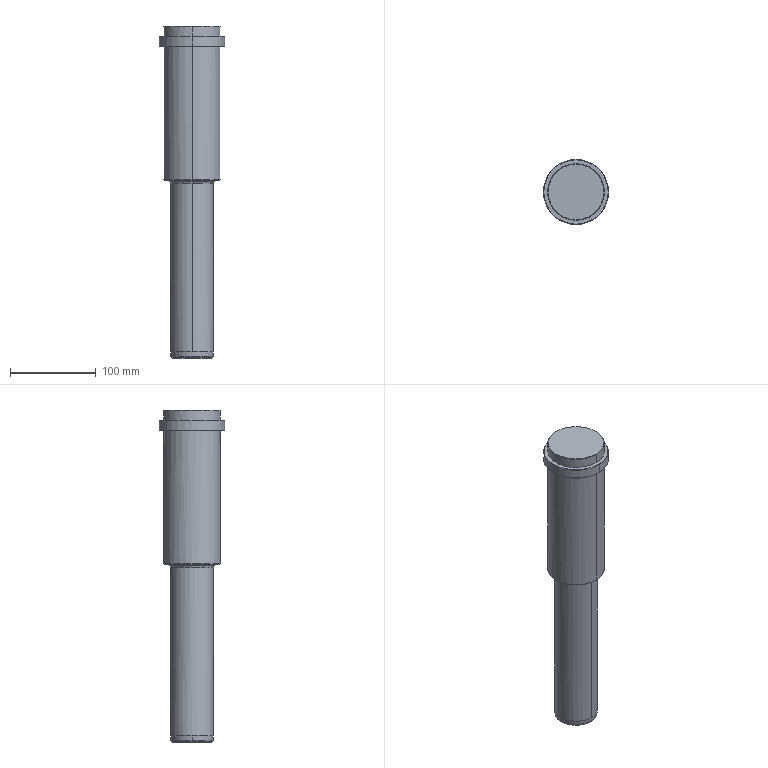Part | Creo | 1 solid | 31 faces | box 76 x 76 x 387 mm | volume 1035650 mm3 | cone 10 | cylinder 8 | torus 8 | plane 5 | commonest cylinder face diameters 66 x4 50 x2 76 x2
STEP:
#1=CARTESIAN_POINT('',(255.,259.495,177.));
#2=VERTEX_POINT('',#1);
#3=CARTESIAN_POINT('',(287.5,291.995,177.));
#4=VERTEX_POINT('',#3);
#5=CARTESIAN_POINT('',(255.,291.995,177.));
#6=DIRECTION('',(0.,0.,1.));
#7=DIRECTION('',(0.,-1.,0.));
#8=AXIS2_PLACEMENT_3D('',#5,#6,#7);
#9=CIRCLE('',#8,32.5);
#10=EDGE_CURVE('',#2,#4,#9,.T.);
#11=ORIENTED_EDGE('',*,*,#10,.F.);
#12=CARTESIAN_POINT('',(222.5,291.995,177.));
#13=VERTEX_POINT('',#12);
#14=CARTESIAN_POINT('',(255.,291.995,177.));
#15=DIRECTION('',(0.,0.,1.));
#16=DIRECTION('',(-1.,0.,0.));
#17=AXIS2_PLACEMENT_3D('',#14,#15,#16);
#18=CIRCLE('',#17,32.5);
#19=EDGE_CURVE('',#13,#2,#18,.T.);
#20=ORIENTED_EDGE('',*,*,#19,.F.);
#21=CARTESIAN_POINT('',(255.,324.495,177.));
#22=VERTEX_POINT('',#21);
#23=CARTESIAN_POINT('',(255.,291.995,177.));
#24=DIRECTION('',(0.,0.,1.));
#25=DIRECTION('',(0.,1.,0.));
#26=AXIS2_PLACEMENT_3D('',#23,#24,#25);
#27=CIRCLE('',#26,32.5);
#28=EDGE_CURVE('',#22,#13,#27,.T.);
#29=ORIENTED_EDGE('',*,*,#28,.F.);
#30=CARTESIAN_POINT('',(255.,291.995,177.));
#31=DIRECTION('',(0.,0.,1.));
#32=DIRECTION('',(1.,0.,0.));
#33=AXIS2_PLACEMENT_3D('',#30,#31,#32);
#34=CIRCLE('',#33,32.5);
#35=EDGE_CURVE('',#4,#22,#34,.T.);
#36=ORIENTED_EDGE('',*,*,#35,.F.);
#37=EDGE_LOOP('',(#11,#20,#29,#36));
#38=FACE_OUTER_BOUND('',#37,.F.);
#39=CARTESIAN_POINT('',(65.,43.995,177.));
#40=DIRECTION('',(0.,0.,1.));
#41=DIRECTION('',(0.,-1.,0.));
#42=AXIS2_PLACEMENT_3D('',#39,#40,#41);
#43=PLANE('',#42);
#44=ADVANCED_FACE('',(#38),#43,.T.);
#45=CARTESIAN_POINT('',(255.,258.995,176.5));
#46=VERTEX_POINT('',#45);
#47=CARTESIAN_POINT('',(288.,291.995,176.5));
#48=VERTEX_POINT('',#47);
#49=CARTESIAN_POINT('',(255.,291.995,176.5));
#50=DIRECTION('',(0.,0.,1.));
#51=DIRECTION('',(0.,-1.,0.));
#52=AXIS2_PLACEMENT_3D('',#49,#50,#51);
#53=CIRCLE('',#52,33.);
#54=EDGE_CURVE('',#46,#48,#53,.T.);
#55=ORIENTED_EDGE('',*,*,#54,.F.);
#56=CARTESIAN_POINT('',(222.,291.995,176.5));
#57=VERTEX_POINT('',#56);
#58=CARTESIAN_POINT('',(255.,291.995,176.5));
#59=DIRECTION('',(0.,0.,1.));
#60=DIRECTION('',(-1.,0.,0.));
#61=AXIS2_PLACEMENT_3D('',#58,#59,#60);
#62=CIRCLE('',#61,33.);
#63=EDGE_CURVE('',#57,#46,#62,.T.);
#64=ORIENTED_EDGE('',*,*,#63,.F.);
#65=CARTESIAN_POINT('',(222.5,291.995,177.));
#66=DIRECTION('',(-0.7071,0.,-0.7071));
#67=VECTOR('',#66,0.7071);
#68=LINE('',#65,#67);
#69=EDGE_CURVE('',#13,#57,#68,.T.);
#70=ORIENTED_EDGE('',*,*,#69,.F.);
#71=ORIENTED_EDGE('',*,*,#19,.T.);
#72=ORIENTED_EDGE('',*,*,#10,.T.);
#73=CARTESIAN_POINT('',(287.5,291.995,177.));
#74=DIRECTION('',(0.7071,0.,-0.7071));
#75=VECTOR('',#74,0.7071);
#76=LINE('',#73,#75);
#77=EDGE_CURVE('',#4,#48,#76,.T.);
#78=ORIENTED_EDGE('',*,*,#77,.T.);
#79=EDGE_LOOP('',(#55,#64,#70,#71,#72,#78));
#80=FACE_OUTER_BOUND('',#79,.F.);
#81=CARTESIAN_POINT('',(255.,291.995,176.75));
#82=DIRECTION('',(0.,0.,-1.));
#83=DIRECTION('',(-1.,0.,0.));
#84=AXIS2_PLACEMENT_3D('',#81,#82,#83);
#85=CONICAL_SURFACE('',#84,32.75,45.);
#86=ADVANCED_FACE('',(#80),#85,.T.);
#87=CARTESIAN_POINT('',(255.,324.995,176.5));
#88=VERTEX_POINT('',#87);
#89=CARTESIAN_POINT('',(255.,291.995,176.5));
#90=DIRECTION('',(0.,0.,1.));
#91=DIRECTION('',(1.,0.,0.));
#92=AXIS2_PLACEMENT_3D('',#89,#90,#91);
#93=CIRCLE('',#92,33.);
#94=EDGE_CURVE('',#48,#88,#93,.T.);
#95=ORIENTED_EDGE('',*,*,#94,.T.);
#96=CARTESIAN_POINT('',(255.,324.995,165.));
#97=VERTEX_POINT('',#96);
#98=CARTESIAN_POINT('',(255.,324.995,165.));
#99=DIRECTION('',(0.,0.,1.));
#100=VECTOR('',#99,11.5);
#101=LINE('',#98,#100);
#102=EDGE_CURVE('',#97,#88,#101,.T.);
#103=ORIENTED_EDGE('',*,*,#102,.F.);
#104=CARTESIAN_POINT('',(255.,258.995,165.));
#105=VERTEX_POINT('',#104);
#106=CARTESIAN_POINT('',(255.,291.995,165.));
#107=DIRECTION('',(0.,0.,-1.));
#108=DIRECTION('',(0.,1.,0.));
#109=AXIS2_PLACEMENT_3D('',#106,#107,#108);
#110=CIRCLE('',#109,33.);
#111=EDGE_CURVE('',#97,#105,#110,.T.);
#112=ORIENTED_EDGE('',*,*,#111,.T.);
#113=CARTESIAN_POINT('',(255.,258.995,165.));
#114=DIRECTION('',(0.,0.,1.));
#115=VECTOR('',#114,11.5);
#116=LINE('',#113,#115);
#117=EDGE_CURVE('',#105,#46,#116,.T.);
#118=ORIENTED_EDGE('',*,*,#117,.T.);
#119=ORIENTED_EDGE('',*,*,#54,.T.);
#120=EDGE_LOOP('',(#95,#103,#112,#118,#119));
#121=FACE_OUTER_BOUND('',#120,.F.);
#122=CARTESIAN_POINT('',(255.,291.995,165.));
#123=DIRECTION('',(0.,0.,1.));
#124=DIRECTION('',(0.,-1.,0.));
#125=AXIS2_PLACEMENT_3D('',#122,#123,#124);
#126=CYLINDRICAL_SURFACE('',#125,33.);
#127=ADVANCED_FACE('',(#121),#126,.T.);
#128=ORIENTED_EDGE('',*,*,#94,.F.);
#129=ORIENTED_EDGE('',*,*,#77,.F.);
#130=ORIENTED_EDGE('',*,*,#35,.T.);
#131=ORIENTED_EDGE('',*,*,#28,.T.);
#132=ORIENTED_EDGE('',*,*,#69,.T.);
#133=CARTESIAN_POINT('',(255.,291.995,176.5));
#134=DIRECTION('',(0.,0.,1.));
#135=DIRECTION('',(0.,1.,0.));
#136=AXIS2_PLACEMENT_3D('',#133,#134,#135);
#137=CIRCLE('',#136,33.);
#138=EDGE_CURVE('',#88,#57,#137,.T.);
#139=ORIENTED_EDGE('',*,*,#138,.F.);
#140=EDGE_LOOP('',(#128,#129,#130,#131,#132,#139));
#141=FACE_OUTER_BOUND('',#140,.F.);
#142=CARTESIAN_POINT('',(255.,291.995,176.75));
#143=DIRECTION('',(0.,0.,-1.));
#144=DIRECTION('',(-1.,0.,0.));
#145=AXIS2_PLACEMENT_3D('',#142,#143,#144);
#146=CONICAL_SURFACE('',#145,32.75,45.);
#147=ADVANCED_FACE('',(#141),#146,.T.);
#148=ORIENTED_EDGE('',*,*,#63,.T.);
#149=ORIENTED_EDGE('',*,*,#117,.F.);
#150=CARTESIAN_POINT('',(255.,291.995,165.));
#151=DIRECTION('',(0.,0.,-1.));
#152=DIRECTION('',(0.,-1.,0.));
#153=AXIS2_PLACEMENT_3D('',#150,#151,#152);
#154=CIRCLE('',#153,33.);
#155=EDGE_CURVE('',#105,#97,#154,.T.);
#156=ORIENTED_EDGE('',*,*,#155,.T.);
#157=ORIENTED_EDGE('',*,*,#102,.T.);
#158=ORIENTED_EDGE('',*,*,#138,.T.);
#159=EDGE_LOOP('',(#148,#149,#156,#157,#158));
#160=FACE_OUTER_BOUND('',#159,.F.);
#161=CARTESIAN_POINT('',(255.,291.995,165.));
#162=DIRECTION('',(0.,0.,1.));
#163=DIRECTION('',(0.,-1.,0.));
#164=AXIS2_PLACEMENT_3D('',#161,#162,#163);
#165=CYLINDRICAL_SURFACE('',#164,33.);
#166=ADVANCED_FACE('',(#160),#165,.T.);
#167=CARTESIAN_POINT('',(255.,254.495,165.));
#168=VERTEX_POINT('',#167);
#169=CARTESIAN_POINT('',(292.5,291.995,165.));
#170=VERTEX_POINT('',#169);
#171=CARTESIAN_POINT('',(255.,291.995,165.));
#172=DIRECTION('',(0.,0.,1.));
#173=DIRECTION('',(0.,-1.,0.));
#174=AXIS2_PLACEMENT_3D('',#171,#172,#173);
#175=CIRCLE('',#174,37.5);
#176=EDGE_CURVE('',#168,#170,#175,.T.);
#177=ORIENTED_EDGE('',*,*,#176,.F.);
#178=CARTESIAN_POINT('',(217.5,291.995,165.));
#179=VERTEX_POINT('',#178);
#180=CARTESIAN_POINT('',(255.,291.995,165.));
#181=DIRECTION('',(0.,0.,1.));
#182=DIRECTION('',(-1.,0.,0.));
#183=AXIS2_PLACEMENT_3D('',#180,#181,#182);
#184=CIRCLE('',#183,37.5);
#185=EDGE_CURVE('',#179,#168,#184,.T.);
#186=ORIENTED_EDGE('',*,*,#185,.F.);
#187=CARTESIAN_POINT('',(255.,329.495,165.));
#188=VERTEX_POINT('',#187);
#189=CARTESIAN_POINT('',(255.,291.995,165.));
#190=DIRECTION('',(0.,0.,1.));
#191=DIRECTION('',(0.,1.,0.));
#192=AXIS2_PLACEMENT_3D('',#189,#190,#191);
#193=CIRCLE('',#192,37.5);
#194=EDGE_CURVE('',#188,#179,#193,.T.);
#195=ORIENTED_EDGE('',*,*,#194,.F.);
#196=CARTESIAN_POINT('',(255.,291.995,165.));
#197=DIRECTION('',(0.,0.,1.));
#198=DIRECTION('',(1.,0.,0.));
#199=AXIS2_PLACEMENT_3D('',#196,#197,#198);
#200=CIRCLE('',#199,37.5);
#201=EDGE_CURVE('',#170,#188,#200,.T.);
#202=ORIENTED_EDGE('',*,*,#201,.F.);
#203=EDGE_LOOP('',(#177,#186,#195,#202));
#204=FACE_OUTER_BOUND('',#203,.F.);
#205=ORIENTED_EDGE('',*,*,#155,.F.);
#206=ORIENTED_EDGE('',*,*,#111,.F.);
#207=EDGE_LOOP('',(#205,#206));
#208=FACE_BOUND('',#207,.F.);
#209=CARTESIAN_POINT('',(-210.,43.995,165.));
#210=DIRECTION('',(0.,0.,-1.));
#211=DIRECTION('',(0.,1.,0.));
#212=AXIS2_PLACEMENT_3D('',#209,#210,#211);
#213=PLANE('',#212);
#214=ADVANCED_FACE('',(#204,#208),#213,.F.);
#215=CARTESIAN_POINT('',(255.,253.995,164.5));
#216=VERTEX_POINT('',#215);
#217=CARTESIAN_POINT('',(293.,291.995,164.5));
#218=VERTEX_POINT('',#217);
#219=CARTESIAN_POINT('',(255.,291.995,164.5));
#220=DIRECTION('',(0.,0.,1.));
#221=DIRECTION('',(0.,-1.,0.));
#222=AXIS2_PLACEMENT_3D('',#219,#220,#221);
#223=CIRCLE('',#222,38.);
#224=EDGE_CURVE('',#216,#218,#223,.T.);
#225=ORIENTED_EDGE('',*,*,#224,.F.);
#226=CARTESIAN_POINT('',(217.,291.995,164.5));
#227=VERTEX_POINT('',#226);
#228=CARTESIAN_POINT('',(255.,291.995,164.5));
#229=DIRECTION('',(0.,0.,1.));
#230=DIRECTION('',(-1.,0.,0.));
#231=AXIS2_PLACEMENT_3D('',#228,#229,#230);
#232=CIRCLE('',#231,38.);
#233=EDGE_CURVE('',#227,#216,#232,.T.);
#234=ORIENTED_EDGE('',*,*,#233,.F.);
#235=CARTESIAN_POINT('',(217.5,291.995,165.));
#236=DIRECTION('',(-0.7071,0.,-0.7071));
#237=VECTOR('',#236,0.7071);
#238=LINE('',#235,#237);
#239=EDGE_CURVE('',#179,#227,#238,.T.);
#240=ORIENTED_EDGE('',*,*,#239,.F.);
#241=ORIENTED_EDGE('',*,*,#185,.T.);
#242=ORIENTED_EDGE('',*,*,#176,.T.);
#243=CARTESIAN_POINT('',(292.5,291.995,165.));
#244=DIRECTION('',(0.7071,0.,-0.7071));
#245=VECTOR('',#244,0.7071);
#246=LINE('',#243,#245);
#247=EDGE_CURVE('',#170,#218,#246,.T.);
#248=ORIENTED_EDGE('',*,*,#247,.T.);
#249=EDGE_LOOP('',(#225,#234,#240,#241,#242,#248));
#250=FACE_OUTER_BOUND('',#249,.F.);
#251=CARTESIAN_POINT('',(255.,291.995,164.75));
#252=DIRECTION('',(0.,0.,-1.));
#253=DIRECTION('',(-1.,0.,0.));
#254=AXIS2_PLACEMENT_3D('',#251,#252,#253);
#255=CONICAL_SURFACE('',#254,37.75,45.);
#256=ADVANCED_FACE('',(#250),#255,.T.);
#257=CARTESIAN_POINT('',(293.,291.995,153.5));
#258=VERTEX_POINT('',#257);
#259=CARTESIAN_POINT('',(255.,253.995,153.5));
#260=VERTEX_POINT('',#259);
#261=CARTESIAN_POINT('',(255.,291.995,153.5));
#262=DIRECTION('',(0.,0.,-1.));
#263=DIRECTION('',(1.,0.,0.));
#264=AXIS2_PLACEMENT_3D('',#261,#262,#263);
#265=CIRCLE('',#264,38.);
#266=EDGE_CURVE('',#258,#260,#265,.T.);
#267=ORIENTED_EDGE('',*,*,#266,.T.);
#268=CARTESIAN_POINT('',(255.,253.995,153.5));
#269=DIRECTION('',(0.,0.,1.));
#270=VECTOR('',#269,11.);
#271=LINE('',#268,#270);
#272=EDGE_CURVE('',#260,#216,#271,.T.);
#273=ORIENTED_EDGE('',*,*,#272,.T.);
#274=ORIENTED_EDGE('',*,*,#224,.T.);
#275=CARTESIAN_POINT('',(255.,329.995,164.5));
#276=VERTEX_POINT('',#275);
#277=CARTESIAN_POINT('',(255.,291.995,164.5));
#278=DIRECTION('',(0.,0.,1.));
#279=DIRECTION('',(1.,0.,0.));
#280=AXIS2_PLACEMENT_3D('',#277,#278,#279);
#281=CIRCLE('',#280,38.);
#282=EDGE_CURVE('',#218,#276,#281,.T.);
#283=ORIENTED_EDGE('',*,*,#282,.T.);
#284=CARTESIAN_POINT('',(255.,329.995,153.5));
#285=VERTEX_POINT('',#284);
#286=CARTESIAN_POINT('',(255.,329.995,153.5));
#287=DIRECTION('',(0.,0.,1.));
#288=VECTOR('',#287,11.);
#289=LINE('',#286,#288);
#290=EDGE_CURVE('',#285,#276,#289,.T.);
#291=ORIENTED_EDGE('',*,*,#290,.F.);
#292=CARTESIAN_POINT('',(255.,291.995,153.5));
#293=DIRECTION('',(0.,0.,-1.));
#294=DIRECTION('',(0.,1.,0.));
#295=AXIS2_PLACEMENT_3D('',#292,#293,#294);
#296=CIRCLE('',#295,38.);
#297=EDGE_CURVE('',#285,#258,#296,.T.);
#298=ORIENTED_EDGE('',*,*,#297,.T.);
#299=EDGE_LOOP('',(#267,#273,#274,#283,#291,#298));
#300=FACE_OUTER_BOUND('',#299,.F.);
#301=CARTESIAN_POINT('',(255.,291.995,165.));
#302=DIRECTION('',(0.,0.,1.));
#303=DIRECTION('',(0.,-1.,0.));
#304=AXIS2_PLACEMENT_3D('',#301,#302,#303);
#305=CYLINDRICAL_SURFACE('',#304,38.);
#306=ADVANCED_FACE('',(#300),#305,.T.);
#307=CARTESIAN_POINT('',(217.,291.995,153.5));
#308=VERTEX_POINT('',#307);
#309=CARTESIAN_POINT('',(255.,291.995,153.5));
#310=DIRECTION('',(0.,0.,-1.));
#311=DIRECTION('',(0.,-1.,0.));
#312=AXIS2_PLACEMENT_3D('',#309,#310,#311);
#313=CIRCLE('',#312,38.);
#314=EDGE_CURVE('',#260,#308,#313,.T.);
#315=ORIENTED_EDGE('',*,*,#314,.F.);
#316=ORIENTED_EDGE('',*,*,#266,.F.);
#317=CARTESIAN_POINT('',(292.5,291.995,153.));
#318=VERTEX_POINT('',#317);
#319=CARTESIAN_POINT('',(292.5,291.995,153.));
#320=DIRECTION('',(0.7071,0.,0.7071));
#321=VECTOR('',#320,0.7071);
#322=LINE('',#319,#321);
#323=EDGE_CURVE('',#318,#258,#322,.T.);
#324=ORIENTED_EDGE('',*,*,#323,.F.);
#325=CARTESIAN_POINT('',(255.,254.495,153.));
#326=VERTEX_POINT('',#325);
#327=CARTESIAN_POINT('',(255.,291.995,153.));
#328=DIRECTION('',(0.,0.,-1.));
#329=DIRECTION('',(1.,0.,0.));
#330=AXIS2_PLACEMENT_3D('',#327,#328,#329);
#331=CIRCLE('',#330,37.5);
#332=EDGE_CURVE('',#318,#326,#331,.T.);
#333=ORIENTED_EDGE('',*,*,#332,.T.);
#334=CARTESIAN_POINT('',(217.5,291.995,153.));
#335=VERTEX_POINT('',#334);
#336=CARTESIAN_POINT('',(255.,291.995,153.));
#337=DIRECTION('',(0.,0.,-1.));
#338=DIRECTION('',(0.,-1.,0.));
#339=AXIS2_PLACEMENT_3D('',#336,#337,#338);
#340=CIRCLE('',#339,37.5);
#341=EDGE_CURVE('',#326,#335,#340,.T.);
#342=ORIENTED_EDGE('',*,*,#341,.T.);
#343=CARTESIAN_POINT('',(217.5,291.995,153.));
#344=DIRECTION('',(-0.7071,0.,0.7071));
#345=VECTOR('',#344,0.7071);
#346=LINE('',#343,#345);
#347=EDGE_CURVE('',#335,#308,#346,.T.);
#348=ORIENTED_EDGE('',*,*,#347,.T.);
#349=EDGE_LOOP('',(#315,#316,#324,#333,#342,#348));
#350=FACE_OUTER_BOUND('',#349,.F.);
#351=CARTESIAN_POINT('',(255.,291.995,153.25));
#352=DIRECTION('',(0.,0.,1.));
#353=DIRECTION('',(-1.,0.,0.));
#354=AXIS2_PLACEMENT_3D('',#351,#352,#353);
#355=CONICAL_SURFACE('',#354,37.75,45.);
#356=ADVANCED_FACE('',(#350),#355,.T.);
#357=CARTESIAN_POINT('',(255.,291.995,153.5));
#358=DIRECTION('',(0.,0.,-1.));
#359=DIRECTION('',(-1.,0.,0.));
#360=AXIS2_PLACEMENT_3D('',#357,#358,#359);
#361=CIRCLE('',#360,38.);
#362=EDGE_CURVE('',#308,#285,#361,.T.);
#363=ORIENTED_EDGE('',*,*,#362,.T.);
#364=ORIENTED_EDGE('',*,*,#290,.T.);
#365=CARTESIAN_POINT('',(255.,291.995,164.5));
#366=DIRECTION('',(0.,0.,1.));
#367=DIRECTION('',(0.,1.,0.));
#368=AXIS2_PLACEMENT_3D('',#365,#366,#367);
#369=CIRCLE('',#368,38.);
#370=EDGE_CURVE('',#276,#227,#369,.T.);
#371=ORIENTED_EDGE('',*,*,#370,.T.);
#372=ORIENTED_EDGE('',*,*,#233,.T.);
#373=ORIENTED_EDGE('',*,*,#272,.F.);
#374=ORIENTED_EDGE('',*,*,#314,.T.);
#375=EDGE_LOOP('',(#363,#364,#371,#372,#373,#374));
#376=FACE_OUTER_BOUND('',#375,.F.);
#377=CARTESIAN_POINT('',(255.,291.995,165.));
#378=DIRECTION('',(0.,0.,1.));
#379=DIRECTION('',(0.,-1.,0.));
#380=AXIS2_PLACEMENT_3D('',#377,#378,#379);
#381=CYLINDRICAL_SURFACE('',#380,38.);
#382=ADVANCED_FACE('',(#376),#381,.T.);
#383=ORIENTED_EDGE('',*,*,#362,.F.);
#384=ORIENTED_EDGE('',*,*,#347,.F.);
#385=CARTESIAN_POINT('',(255.,329.495,153.));
#386=VERTEX_POINT('',#385);
#387=CARTESIAN_POINT('',(255.,291.995,153.));
#388=DIRECTION('',(0.,0.,-1.));
#389=DIRECTION('',(-1.,0.,0.));
#390=AXIS2_PLACEMENT_3D('',#387,#388,#389);
#391=CIRCLE('',#390,37.5);
#392=EDGE_CURVE('',#335,#386,#391,.T.);
#393=ORIENTED_EDGE('',*,*,#392,.T.);
#394=CARTESIAN_POINT('',(255.,291.995,153.));
#395=DIRECTION('',(0.,0.,-1.));
#396=DIRECTION('',(0.,1.,0.));
#397=AXIS2_PLACEMENT_3D('',#394,#395,#396);
#398=CIRCLE('',#397,37.5);
#399=EDGE_CURVE('',#386,#318,#398,.T.);
#400=ORIENTED_EDGE('',*,*,#399,.T.);
#401=ORIENTED_EDGE('',*,*,#323,.T.);
#402=ORIENTED_EDGE('',*,*,#297,.F.);
#403=EDGE_LOOP('',(#383,#384,#393,#400,#401,#402));
#404=FACE_OUTER_BOUND('',#403,.F.);
#405=CARTESIAN_POINT('',(255.,291.995,153.25));
#406=DIRECTION('',(0.,0.,1.));
#407=DIRECTION('',(-1.,0.,0.));
#408=AXIS2_PLACEMENT_3D('',#405,#406,#407);
#409=CONICAL_SURFACE('',#408,37.75,45.);
#410=ADVANCED_FACE('',(#404),#409,.T.);
#411=ORIENTED_EDGE('',*,*,#341,.F.);
#412=ORIENTED_EDGE('',*,*,#332,.F.);
#413=ORIENTED_EDGE('',*,*,#399,.F.);
#414=ORIENTED_EDGE('',*,*,#392,.F.);
#415=EDGE_LOOP('',(#411,#412,#413,#414));
#416=FACE_OUTER_BOUND('',#415,.F.);
#417=CARTESIAN_POINT('',(255.,324.995,153.));
#418=VERTEX_POINT('',#417);
#419=CARTESIAN_POINT('',(255.,258.995,153.));
#420=VERTEX_POINT('',#419);
#421=CARTESIAN_POINT('',(255.,291.995,153.));
#422=DIRECTION('',(0.,0.,1.));
#423=DIRECTION('',(0.,1.,0.));
#424=AXIS2_PLACEMENT_3D('',#421,#422,#423);
#425=CIRCLE('',#424,33.);
#426=EDGE_CURVE('',#418,#420,#425,.T.);
#427=ORIENTED_EDGE('',*,*,#426,.F.);
#428=CARTESIAN_POINT('',(255.,291.995,153.));
#429=DIRECTION('',(0.,0.,1.));
#430=DIRECTION('',(0.,-1.,0.));
#431=AXIS2_PLACEMENT_3D('',#428,#429,#430);
#432=CIRCLE('',#431,33.);
#433=EDGE_CURVE('',#420,#418,#432,.T.);
#434=ORIENTED_EDGE('',*,*,#433,.F.);
#435=EDGE_LOOP('',(#427,#434));
#436=FACE_BOUND('',#435,.F.);
#437=CARTESIAN_POINT('',(65.,43.995,153.));
#438=DIRECTION('',(0.,0.,1.));
#439=DIRECTION('',(0.,-1.,0.));
#440=AXIS2_PLACEMENT_3D('',#437,#438,#439);
#441=PLANE('',#440);
#442=ADVANCED_FACE('',(#416,#436),#441,.F.);
#443=ORIENTED_EDGE('',*,*,#426,.T.);
#444=CARTESIAN_POINT('',(255.,258.995,-2.5));
#445=VERTEX_POINT('',#444);
#446=CARTESIAN_POINT('',(255.,258.995,153.));
#447=DIRECTION('',(0.,0.,-1.));
#448=VECTOR('',#447,155.5);
#449=LINE('',#446,#448);
#450=EDGE_CURVE('',#420,#445,#449,.T.);
#451=ORIENTED_EDGE('',*,*,#450,.T.);
#452=CARTESIAN_POINT('',(222.,291.995,-2.5));
#453=VERTEX_POINT('',#452);
#454=CARTESIAN_POINT('',(255.,291.995,-2.5));
#455=DIRECTION('',(0.,0.,-1.));
#456=DIRECTION('',(0.,-1.,0.));
#457=AXIS2_PLACEMENT_3D('',#454,#455,#456);
#458=CIRCLE('',#457,33.);
#459=EDGE_CURVE('',#445,#453,#458,.T.);
#460=ORIENTED_EDGE('',*,*,#459,.T.);
#461=CARTESIAN_POINT('',(255.,324.995,-2.5));
#462=VERTEX_POINT('',#461);
#463=CARTESIAN_POINT('',(255.,291.995,-2.5));
#464=DIRECTION('',(0.,0.,-1.));
#465=DIRECTION('',(-1.,0.,0.));
#466=AXIS2_PLACEMENT_3D('',#463,#464,#465);
#467=CIRCLE('',#466,33.);
#468=EDGE_CURVE('',#453,#462,#467,.T.);
#469=ORIENTED_EDGE('',*,*,#468,.T.);
#470=CARTESIAN_POINT('',(255.,324.995,153.));
#471=DIRECTION('',(0.,0.,-1.));
#472=VECTOR('',#471,155.5);
#473=LINE('',#470,#472);
#474=EDGE_CURVE('',#418,#462,#473,.T.);
#475=ORIENTED_EDGE('',*,*,#474,.F.);
#476=EDGE_LOOP('',(#443,#451,#460,#469,#475));
#477=FACE_OUTER_BOUND('',#476,.F.);
#478=CARTESIAN_POINT('',(255.,291.995,153.));
#479=DIRECTION('',(0.,0.,-1.));
#480=DIRECTION('',(0.,1.,0.));
#481=AXIS2_PLACEMENT_3D('',#478,#479,#480);
#482=CYLINDRICAL_SURFACE('',#481,33.);
#483=ADVANCED_FACE('',(#477),#482,.T.);
#484=ORIENTED_EDGE('',*,*,#433,.T.);
#485=ORIENTED_EDGE('',*,*,#474,.T.);
#486=CARTESIAN_POINT('',(288.,291.995,-2.5));
#487=VERTEX_POINT('',#486);
#488=CARTESIAN_POINT('',(255.,291.995,-2.5));
#489=DIRECTION('',(0.,0.,-1.));
#490=DIRECTION('',(0.,1.,0.));
#491=AXIS2_PLACEMENT_3D('',#488,#489,#490);
#492=CIRCLE('',#491,33.);
#493=EDGE_CURVE('',#462,#487,#492,.T.);
#494=ORIENTED_EDGE('',*,*,#493,.T.);
#495=CARTESIAN_POINT('',(255.,291.995,-2.5));
#496=DIRECTION('',(0.,0.,-1.));
#497=DIRECTION('',(1.,0.,0.));
#498=AXIS2_PLACEMENT_3D('',#495,#496,#497);
#499=CIRCLE('',#498,33.);
#500=EDGE_CURVE('',#487,#445,#499,.T.);
#501=ORIENTED_EDGE('',*,*,#500,.T.);
#502=ORIENTED_EDGE('',*,*,#450,.F.);
#503=EDGE_LOOP('',(#484,#485,#494,#501,#502));
#504=FACE_OUTER_BOUND('',#503,.F.);
#505=CARTESIAN_POINT('',(255.,291.995,153.));
#506=DIRECTION('',(0.,0.,-1.));
#507=DIRECTION('',(0.,1.,0.));
#508=AXIS2_PLACEMENT_3D('',#505,#506,#507);
#509=CYLINDRICAL_SURFACE('',#508,33.);
#510=ADVANCED_FACE('',(#504),#509,.T.);
#511=ORIENTED_EDGE('',*,*,#468,.F.);
#512=CARTESIAN_POINT('',(222.5,291.995,-3.));
#513=VERTEX_POINT('',#512);
#514=CARTESIAN_POINT('',(222.5,291.995,-3.));
#515=DIRECTION('',(-0.7071,0.,0.7071));
#516=VECTOR('',#515,0.7071);
#517=LINE('',#514,#516);
#518=EDGE_CURVE('',#513,#453,#517,.T.);
#519=ORIENTED_EDGE('',*,*,#518,.F.);
#520=CARTESIAN_POINT('',(255.,324.495,-3.));
#521=VERTEX_POINT('',#520);
#522=CARTESIAN_POINT('',(255.,291.995,-3.));
#523=DIRECTION('',(0.,0.,-1.));
#524=DIRECTION('',(-1.,0.,0.));
#525=AXIS2_PLACEMENT_3D('',#522,#523,#524);
#526=CIRCLE('',#525,32.5);
#527=EDGE_CURVE('',#513,#521,#526,.T.);
#528=ORIENTED_EDGE('',*,*,#527,.T.);
#529=CARTESIAN_POINT('',(287.5,291.995,-3.));
#530=VERTEX_POINT('',#529);
#531=CARTESIAN_POINT('',(255.,291.995,-3.));
#532=DIRECTION('',(0.,0.,-1.));
#533=DIRECTION('',(0.,1.,0.));
#534=AXIS2_PLACEMENT_3D('',#531,#532,#533);
#535=CIRCLE('',#534,32.5);
#536=EDGE_CURVE('',#521,#530,#535,.T.);
#537=ORIENTED_EDGE('',*,*,#536,.T.);
#538=CARTESIAN_POINT('',(287.5,291.995,-3.));
#539=DIRECTION('',(0.7071,0.,0.7071));
#540=VECTOR('',#539,0.7071);
#541=LINE('',#538,#540);
#542=EDGE_CURVE('',#530,#487,#541,.T.);
#543=ORIENTED_EDGE('',*,*,#542,.T.);
#544=ORIENTED_EDGE('',*,*,#493,.F.);
#545=EDGE_LOOP('',(#511,#519,#528,#537,#543,#544));
#546=FACE_OUTER_BOUND('',#545,.F.);
#547=CARTESIAN_POINT('',(255.,291.995,-2.75));
#548=DIRECTION('',(0.,0.,1.));
#549=DIRECTION('',(-1.,0.,0.));
#550=AXIS2_PLACEMENT_3D('',#547,#548,#549);
#551=CONICAL_SURFACE('',#550,32.75,45.);
#552=ADVANCED_FACE('',(#546),#551,.T.);
#553=ORIENTED_EDGE('',*,*,#459,.F.);
#554=ORIENTED_EDGE('',*,*,#500,.F.);
#555=ORIENTED_EDGE('',*,*,#542,.F.);
#556=CARTESIAN_POINT('',(255.,259.495,-3.));
#557=VERTEX_POINT('',#556);
#558=CARTESIAN_POINT('',(255.,291.995,-3.));
#559=DIRECTION('',(0.,0.,-1.));
#560=DIRECTION('',(1.,0.,0.));
#561=AXIS2_PLACEMENT_3D('',#558,#559,#560);
#562=CIRCLE('',#561,32.5);
#563=EDGE_CURVE('',#530,#557,#562,.T.);
#564=ORIENTED_EDGE('',*,*,#563,.T.);
#565=CARTESIAN_POINT('',(255.,291.995,-3.));
#566=DIRECTION('',(0.,0.,-1.));
#567=DIRECTION('',(0.,-1.,0.));
#568=AXIS2_PLACEMENT_3D('',#565,#566,#567);
#569=CIRCLE('',#568,32.5);
#570=EDGE_CURVE('',#557,#513,#569,.T.);
#571=ORIENTED_EDGE('',*,*,#570,.T.);
#572=ORIENTED_EDGE('',*,*,#518,.T.);
#573=EDGE_LOOP('',(#553,#554,#555,#564,#571,#572));
#574=FACE_OUTER_BOUND('',#573,.F.);
#575=CARTESIAN_POINT('',(255.,291.995,-2.75));
#576=DIRECTION('',(0.,0.,1.));
#577=DIRECTION('',(-1.,0.,0.));
#578=AXIS2_PLACEMENT_3D('',#575,#576,#577);
#579=CONICAL_SURFACE('',#578,32.75,45.);
#580=ADVANCED_FACE('',(#574),#579,.T.);
#581=ORIENTED_EDGE('',*,*,#570,.F.);
#582=ORIENTED_EDGE('',*,*,#563,.F.);
#583=ORIENTED_EDGE('',*,*,#536,.F.);
#584=ORIENTED_EDGE('',*,*,#527,.F.);
#585=EDGE_LOOP('',(#581,#582,#583,#584));
#586=FACE_OUTER_BOUND('',#585,.F.);
#587=CARTESIAN_POINT('',(255.,262.995,-3.));
#588=VERTEX_POINT('',#587);
#589=CARTESIAN_POINT('',(256.472,263.033,-3.));
#590=VERTEX_POINT('',#589);
#591=CARTESIAN_POINT('',(255.,291.995,-3.));
#592=DIRECTION('',(0.,0.,1.));
#593=DIRECTION('',(0.,-1.,0.));
#594=AXIS2_PLACEMENT_3D('',#591,#592,#593);
#595=CIRCLE('',#594,29.);
#596=EDGE_CURVE('',#588,#590,#595,.T.);
#597=ORIENTED_EDGE('',*,*,#596,.F.);
#598=CARTESIAN_POINT('',(253.528,320.958,-3.));
#599=VERTEX_POINT('',#598);
#600=CARTESIAN_POINT('',(255.,291.995,-3.));
#601=DIRECTION('',(0.,0.,1.));
#602=DIRECTION('',(-0.05077,0.9987,0.));
#603=AXIS2_PLACEMENT_3D('',#600,#601,#602);
#604=CIRCLE('',#603,29.);
#605=EDGE_CURVE('',#599,#588,#604,.T.);
#606=ORIENTED_EDGE('',*,*,#605,.F.);
#607=CARTESIAN_POINT('',(255.,291.995,-3.));
#608=DIRECTION('',(0.,0.,1.));
#609=DIRECTION('',(0.05077,-0.9987,0.));
#610=AXIS2_PLACEMENT_3D('',#607,#608,#609);
#611=CIRCLE('',#610,29.);
#612=EDGE_CURVE('',#590,#599,#611,.T.);
#613=ORIENTED_EDGE('',*,*,#612,.F.);
#614=EDGE_LOOP('',(#597,#606,#613));
#615=FACE_BOUND('',#614,.F.);
#616=CARTESIAN_POINT('',(-210.,43.995,-3.));
#617=DIRECTION('',(0.,0.,-1.));
#618=DIRECTION('',(0.,1.,0.));
#619=AXIS2_PLACEMENT_3D('',#616,#617,#618);
#620=PLANE('',#619);
#621=ADVANCED_FACE('',(#586,#615),#620,.T.);
#622=ORIENTED_EDGE('',*,*,#605,.T.);
#623=ORIENTED_EDGE('',*,*,#596,.T.);
#624=CARTESIAN_POINT('',(256.329,265.857,-4.172));
#625=VERTEX_POINT('',#624);
#626=CARTESIAN_POINT('',(256.472,263.033,-7.));
#627=DIRECTION('',(0.9987,0.05077,0.));
#628=DIRECTION('',(-0.0359,0.7062,0.7071));
#629=AXIS2_PLACEMENT_3D('',#626,#627,#628);
#630=CIRCLE('',#629,4.);
#631=EDGE_CURVE('',#625,#590,#630,.T.);
#632=ORIENTED_EDGE('',*,*,#631,.F.);
#633=CARTESIAN_POINT('',(253.671,318.133,-4.172));
#634=VERTEX_POINT('',#633);
#635=CARTESIAN_POINT('',(255.,291.995,-4.172));
#636=DIRECTION('',(0.,0.,-1.));
#637=DIRECTION('',(0.05077,-0.9987,0.));
#638=AXIS2_PLACEMENT_3D('',#635,#636,#637);
#639=CIRCLE('',#638,26.172);
#640=EDGE_CURVE('',#625,#634,#639,.T.);
#641=ORIENTED_EDGE('',*,*,#640,.T.);
#642=CARTESIAN_POINT('',(253.528,320.958,-7.));
#643=DIRECTION('',(-0.9987,-0.05077,0.));
#644=DIRECTION('',(0.0359,-0.7062,0.7071));
#645=AXIS2_PLACEMENT_3D('',#642,#643,#644);
#646=CIRCLE('',#645,4.);
#647=EDGE_CURVE('',#634,#599,#646,.T.);
#648=ORIENTED_EDGE('',*,*,#647,.T.);
#649=EDGE_LOOP('',(#622,#623,#632,#641,#648));
#650=FACE_OUTER_BOUND('',#649,.F.);
#651=CARTESIAN_POINT('',(255.,291.995,-7.));
#652=DIRECTION('',(0.,0.,-1.));
#653=DIRECTION('',(0.05077,-0.9987,0.));
#654=AXIS2_PLACEMENT_3D('',#651,#652,#653);
#655=TOROIDAL_SURFACE('',#654,29.,4.);
#656=ADVANCED_FACE('',(#650),#655,.F.);
#657=ORIENTED_EDGE('',*,*,#612,.T.);
#658=ORIENTED_EDGE('',*,*,#647,.F.);
#659=CARTESIAN_POINT('',(255.,291.995,-4.172));
#660=DIRECTION('',(0.,0.,-1.));
#661=DIRECTION('',(-0.05077,0.9987,0.));
#662=AXIS2_PLACEMENT_3D('',#659,#660,#661);
#663=CIRCLE('',#662,26.172);
#664=EDGE_CURVE('',#634,#625,#663,.T.);
#665=ORIENTED_EDGE('',*,*,#664,.T.);
#666=ORIENTED_EDGE('',*,*,#631,.T.);
#667=EDGE_LOOP('',(#657,#658,#665,#666));
#668=FACE_OUTER_BOUND('',#667,.F.);
#669=CARTESIAN_POINT('',(255.,291.995,-7.));
#670=DIRECTION('',(0.,0.,-1.));
#671=DIRECTION('',(0.05077,-0.9987,0.));
#672=AXIS2_PLACEMENT_3D('',#669,#670,#671);
#673=TOROIDAL_SURFACE('',#672,29.,4.);
#674=ADVANCED_FACE('',(#668),#673,.F.);
#675=CARTESIAN_POINT('',(256.269,267.028,-7.));
#676=VERTEX_POINT('',#675);
#677=CARTESIAN_POINT('',(255.,316.995,-7.));
#678=VERTEX_POINT('',#677);
#679=CARTESIAN_POINT('',(255.,291.995,-7.));
#680=DIRECTION('',(0.,0.,1.));
#681=DIRECTION('',(0.05077,-0.9987,0.));
#682=AXIS2_PLACEMENT_3D('',#679,#680,#681);
#683=CIRCLE('',#682,25.);
#684=EDGE_CURVE('',#676,#678,#683,.T.);
#685=ORIENTED_EDGE('',*,*,#684,.F.);
#686=CARTESIAN_POINT('',(256.472,263.033,-7.));
#687=DIRECTION('',(0.9987,0.05077,0.));
#688=DIRECTION('',(-0.05077,0.9987,0.));
#689=AXIS2_PLACEMENT_3D('',#686,#687,#688);
#690=CIRCLE('',#689,4.);
#691=EDGE_CURVE('',#676,#625,#690,.T.);
#692=ORIENTED_EDGE('',*,*,#691,.T.);
#693=ORIENTED_EDGE('',*,*,#664,.F.);
#694=CARTESIAN_POINT('',(253.731,316.963,-7.));
#695=VERTEX_POINT('',#694);
#696=CARTESIAN_POINT('',(253.528,320.958,-7.));
#697=DIRECTION('',(-0.9987,-0.05077,0.));
#698=DIRECTION('',(0.05077,-0.9987,0.));
#699=AXIS2_PLACEMENT_3D('',#696,#697,#698);
#700=CIRCLE('',#699,4.);
#701=EDGE_CURVE('',#695,#634,#700,.T.);
#702=ORIENTED_EDGE('',*,*,#701,.F.);
#703=CARTESIAN_POINT('',(255.,291.995,-7.));
#704=DIRECTION('',(0.,0.,1.));
#705=DIRECTION('',(0.,1.,0.));
#706=AXIS2_PLACEMENT_3D('',#703,#704,#705);
#707=CIRCLE('',#706,25.);
#708=EDGE_CURVE('',#678,#695,#707,.T.);
#709=ORIENTED_EDGE('',*,*,#708,.F.);
#710=EDGE_LOOP('',(#685,#692,#693,#702,#709));
#711=FACE_OUTER_BOUND('',#710,.F.);
#712=CARTESIAN_POINT('',(255.,291.995,-7.));
#713=DIRECTION('',(0.,0.,-1.));
#714=DIRECTION('',(0.05077,-0.9987,0.));
#715=AXIS2_PLACEMENT_3D('',#712,#713,#714);
#716=TOROIDAL_SURFACE('',#715,29.,4.);
#717=ADVANCED_FACE('',(#711),#716,.F.);
#718=ORIENTED_EDGE('',*,*,#684,.T.);
#719=CARTESIAN_POINT('',(255.,316.995,-203.));
#720=VERTEX_POINT('',#719);
#721=CARTESIAN_POINT('',(255.,316.995,-7.));
#722=DIRECTION('',(0.,0.,-1.));
#723=VECTOR('',#722,196.);
#724=LINE('',#721,#723);
#725=EDGE_CURVE('',#678,#720,#724,.T.);
#726=ORIENTED_EDGE('',*,*,#725,.T.);
#727=CARTESIAN_POINT('',(280.,291.995,-203.));
#728=VERTEX_POINT('',#727);
#729=CARTESIAN_POINT('',(255.,291.995,-203.));
#730=DIRECTION('',(0.,0.,-1.));
#731=DIRECTION('',(0.,1.,0.));
#732=AXIS2_PLACEMENT_3D('',#729,#730,#731);
#733=CIRCLE('',#732,25.);
#734=EDGE_CURVE('',#720,#728,#733,.T.);
#735=ORIENTED_EDGE('',*,*,#734,.T.);
#736=CARTESIAN_POINT('',(255.,266.995,-203.));
#737=VERTEX_POINT('',#736);
#738=CARTESIAN_POINT('',(255.,291.995,-203.));
#739=DIRECTION('',(0.,0.,-1.));
#740=DIRECTION('',(1.,0.,0.));
#741=AXIS2_PLACEMENT_3D('',#738,#739,#740);
#742=CIRCLE('',#741,25.);
#743=EDGE_CURVE('',#728,#737,#742,.T.);
#744=ORIENTED_EDGE('',*,*,#743,.T.);
#745=CARTESIAN_POINT('',(255.,266.995,-7.));
#746=VERTEX_POINT('',#745);
#747=CARTESIAN_POINT('',(255.,266.995,-7.));
#748=DIRECTION('',(0.,0.,-1.));
#749=VECTOR('',#748,196.);
#750=LINE('',#747,#749);
#751=EDGE_CURVE('',#746,#737,#750,.T.);
#752=ORIENTED_EDGE('',*,*,#751,.F.);
#753=CARTESIAN_POINT('',(255.,291.995,-7.));
#754=DIRECTION('',(0.,0.,1.));
#755=DIRECTION('',(0.,-1.,0.));
#756=AXIS2_PLACEMENT_3D('',#753,#754,#755);
#757=CIRCLE('',#756,25.);
#758=EDGE_CURVE('',#746,#676,#757,.T.);
#759=ORIENTED_EDGE('',*,*,#758,.T.);
#760=EDGE_LOOP('',(#718,#726,#735,#744,#752,#759));
#761=FACE_OUTER_BOUND('',#760,.F.);
#762=CARTESIAN_POINT('',(255.,291.995,-3.));
#763=DIRECTION('',(0.,0.,-1.));
#764=DIRECTION('',(0.,1.,0.));
#765=AXIS2_PLACEMENT_3D('',#762,#763,#764);
#766=CYLINDRICAL_SURFACE('',#765,25.);
#767=ADVANCED_FACE('',(#761),#766,.T.);
#768=CARTESIAN_POINT('',(255.,291.995,-7.));
#769=DIRECTION('',(0.,0.,1.));
#770=DIRECTION('',(-0.05077,0.9987,0.));
#771=AXIS2_PLACEMENT_3D('',#768,#769,#770);
#772=CIRCLE('',#771,25.);
#773=EDGE_CURVE('',#695,#746,#772,.T.);
#774=ORIENTED_EDGE('',*,*,#773,.T.);
#775=ORIENTED_EDGE('',*,*,#751,.T.);
#776=CARTESIAN_POINT('',(230.,291.995,-203.));
#777=VERTEX_POINT('',#776);
#778=CARTESIAN_POINT('',(255.,291.995,-203.));
#779=DIRECTION('',(0.,0.,-1.));
#780=DIRECTION('',(0.,-1.,0.));
#781=AXIS2_PLACEMENT_3D('',#778,#779,#780);
#782=CIRCLE('',#781,25.);
#783=EDGE_CURVE('',#737,#777,#782,.T.);
#784=ORIENTED_EDGE('',*,*,#783,.T.);
#785=CARTESIAN_POINT('',(255.,291.995,-203.));
#786=DIRECTION('',(0.,0.,-1.));
#787=DIRECTION('',(-1.,0.,0.));
#788=AXIS2_PLACEMENT_3D('',#785,#786,#787);
#789=CIRCLE('',#788,25.);
#790=EDGE_CURVE('',#777,#720,#789,.T.);
#791=ORIENTED_EDGE('',*,*,#790,.T.);
#792=ORIENTED_EDGE('',*,*,#725,.F.);
#793=ORIENTED_EDGE('',*,*,#708,.T.);
#794=EDGE_LOOP('',(#774,#775,#784,#791,#792,#793));
#795=FACE_OUTER_BOUND('',#794,.F.);
#796=CARTESIAN_POINT('',(255.,291.995,-3.));
#797=DIRECTION('',(0.,0.,-1.));
#798=DIRECTION('',(0.,1.,0.));
#799=AXIS2_PLACEMENT_3D('',#796,#797,#798);
#800=CYLINDRICAL_SURFACE('',#799,25.);
#801=ADVANCED_FACE('',(#795),#800,.T.);
#802=ORIENTED_EDGE('',*,*,#758,.F.);
#803=ORIENTED_EDGE('',*,*,#773,.F.);
#804=ORIENTED_EDGE('',*,*,#701,.T.);
#805=ORIENTED_EDGE('',*,*,#640,.F.);
#806=ORIENTED_EDGE('',*,*,#691,.F.);
#807=EDGE_LOOP('',(#802,#803,#804,#805,#806));
#808=FACE_OUTER_BOUND('',#807,.F.);
#809=CARTESIAN_POINT('',(255.,291.995,-7.));
#810=DIRECTION('',(0.,0.,-1.));
#811=DIRECTION('',(0.05077,-0.9987,0.));
#812=AXIS2_PLACEMENT_3D('',#809,#810,#811);
#813=TOROIDAL_SURFACE('',#812,29.,4.);
#814=ADVANCED_FACE('',(#808),#813,.F.);
#815=CARTESIAN_POINT('',(256.791,267.513,-208.174));
#816=VERTEX_POINT('',#815);
#817=CARTESIAN_POINT('',(230.453,291.995,-208.174));
#818=VERTEX_POINT('',#817);
#819=CARTESIAN_POINT('',(255.,291.995,-208.174));
#820=DIRECTION('',(0.,0.,-1.));
#821=DIRECTION('',(0.07298,-0.9973,0.));
#822=AXIS2_PLACEMENT_3D('',#819,#820,#821);
#823=CIRCLE('',#822,24.547);
#824=EDGE_CURVE('',#816,#818,#823,.T.);
#825=ORIENTED_EDGE('',*,*,#824,.T.);
#826=CARTESIAN_POINT('',(230.453,291.995,-208.174));
#827=DIRECTION('',(-0.08716,0.,0.9962));
#828=VECTOR('',#827,5.194);
#829=LINE('',#826,#828);
#830=EDGE_CURVE('',#818,#777,#829,.T.);
#831=ORIENTED_EDGE('',*,*,#830,.T.);
#832=ORIENTED_EDGE('',*,*,#783,.F.);
#833=ORIENTED_EDGE('',*,*,#743,.F.);
#834=CARTESIAN_POINT('',(279.547,291.995,-208.174));
#835=VERTEX_POINT('',#834);
#836=CARTESIAN_POINT('',(279.547,291.995,-208.174));
#837=DIRECTION('',(0.08716,0.,0.9962));
#838=VECTOR('',#837,5.194);
#839=LINE('',#836,#838);
#840=EDGE_CURVE('',#835,#728,#839,.T.);
#841=ORIENTED_EDGE('',*,*,#840,.F.);
#842=CARTESIAN_POINT('',(255.,291.995,-208.174));
#843=DIRECTION('',(0.,0.,-1.));
#844=DIRECTION('',(1.,0.,0.));
#845=AXIS2_PLACEMENT_3D('',#842,#843,#844);
#846=CIRCLE('',#845,24.547);
#847=EDGE_CURVE('',#835,#816,#846,.T.);
#848=ORIENTED_EDGE('',*,*,#847,.T.);
#849=EDGE_LOOP('',(#825,#831,#832,#833,#841,#848));
#850=FACE_OUTER_BOUND('',#849,.F.);
#851=CARTESIAN_POINT('',(255.,291.995,-205.587));
#852=DIRECTION('',(0.,0.,1.));
#853=DIRECTION('',(-1.,0.,0.));
#854=AXIS2_PLACEMENT_3D('',#851,#852,#853);
#855=CONICAL_SURFACE('',#854,24.774,5.);
#856=ADVANCED_FACE('',(#850),#855,.T.);
#857=ORIENTED_EDGE('',*,*,#824,.F.);
#858=CARTESIAN_POINT('',(256.745,268.153,-209.475));
#859=VERTEX_POINT('',#858);
#860=CARTESIAN_POINT('',(256.646,269.501,-208.));
#861=DIRECTION('',(-0.9973,-0.07298,0.));
#862=DIRECTION('',(0.04931,-0.6738,-0.7373));
#863=AXIS2_PLACEMENT_3D('',#860,#861,#862);
#864=CIRCLE('',#863,2.);
#865=EDGE_CURVE('',#859,#816,#864,.T.);
#866=ORIENTED_EDGE('',*,*,#865,.F.);
#867=CARTESIAN_POINT('',(253.255,315.838,-209.475));
#868=VERTEX_POINT('',#867);
#869=CARTESIAN_POINT('',(255.,291.995,-209.475));
#870=DIRECTION('',(0.,0.,1.));
#871=DIRECTION('',(-0.07298,0.9973,0.));
#872=AXIS2_PLACEMENT_3D('',#869,#870,#871);
#873=CIRCLE('',#872,23.906);
#874=EDGE_CURVE('',#868,#859,#873,.T.);
#875=ORIENTED_EDGE('',*,*,#874,.F.);
#876=CARTESIAN_POINT('',(253.209,316.477,-208.174));
#877=VERTEX_POINT('',#876);
#878=CARTESIAN_POINT('',(253.354,314.49,-208.));
#879=DIRECTION('',(0.9973,0.07298,0.));
#880=DIRECTION('',(-0.04931,0.6738,-0.7373));
#881=AXIS2_PLACEMENT_3D('',#878,#879,#880);
#882=CIRCLE('',#881,2.);
#883=EDGE_CURVE('',#868,#877,#882,.T.);
#884=ORIENTED_EDGE('',*,*,#883,.T.);
#885=CARTESIAN_POINT('',(255.,291.995,-208.174));
#886=DIRECTION('',(0.,0.,-1.));
#887=DIRECTION('',(-1.,0.,0.));
#888=AXIS2_PLACEMENT_3D('',#885,#886,#887);
#889=CIRCLE('',#888,24.547);
#890=EDGE_CURVE('',#818,#877,#889,.T.);
#891=ORIENTED_EDGE('',*,*,#890,.F.);
#892=EDGE_LOOP('',(#857,#866,#875,#884,#891));
#893=FACE_OUTER_BOUND('',#892,.F.);
#894=CARTESIAN_POINT('',(255.,291.995,-208.));
#895=DIRECTION('',(0.,0.,1.));
#896=DIRECTION('',(-0.07298,0.9973,0.));
#897=AXIS2_PLACEMENT_3D('',#894,#895,#896);
#898=TOROIDAL_SURFACE('',#897,22.555,2.);
#899=ADVANCED_FACE('',(#893),#898,.T.);
#900=CARTESIAN_POINT('',(255.,316.543,-208.174));
#901=VERTEX_POINT('',#900);
#902=CARTESIAN_POINT('',(255.,291.995,-208.174));
#903=DIRECTION('',(0.,0.,-1.));
#904=DIRECTION('',(-0.00000005,1.,0.));
#905=AXIS2_PLACEMENT_3D('',#902,#903,#904);
#906=CIRCLE('',#905,24.547);
#907=EDGE_CURVE('',#901,#835,#906,.T.);
#908=ORIENTED_EDGE('',*,*,#907,.F.);
#909=CARTESIAN_POINT('',(255.,291.995,-208.174));
#910=DIRECTION('',(0.,0.,-1.));
#911=DIRECTION('',(-0.07298,0.9973,0.));
#912=AXIS2_PLACEMENT_3D('',#909,#910,#911);
#913=CIRCLE('',#912,24.547);
#914=EDGE_CURVE('',#877,#901,#913,.T.);
#915=ORIENTED_EDGE('',*,*,#914,.F.);
#916=ORIENTED_EDGE('',*,*,#883,.F.);
#917=CARTESIAN_POINT('',(255.,291.995,-209.475));
#918=DIRECTION('',(0.,0.,1.));
#919=DIRECTION('',(0.07298,-0.9973,0.));
#920=AXIS2_PLACEMENT_3D('',#917,#918,#919);
#921=CIRCLE('',#920,23.906);
#922=EDGE_CURVE('',#859,#868,#921,.T.);
#923=ORIENTED_EDGE('',*,*,#922,.F.);
#924=ORIENTED_EDGE('',*,*,#865,.T.);
#925=ORIENTED_EDGE('',*,*,#847,.F.);
#926=EDGE_LOOP('',(#908,#915,#916,#923,#924,#925));
#927=FACE_OUTER_BOUND('',#926,.F.);
#928=CARTESIAN_POINT('',(255.,291.995,-208.));
#929=DIRECTION('',(0.,0.,1.));
#930=DIRECTION('',(-0.07298,0.9973,0.));
#931=AXIS2_PLACEMENT_3D('',#928,#929,#930);
#932=TOROIDAL_SURFACE('',#931,22.555,2.);
#933=ADVANCED_FACE('',(#927),#932,.T.);
#934=ORIENTED_EDGE('',*,*,#914,.T.);
#935=ORIENTED_EDGE('',*,*,#907,.T.);
#936=ORIENTED_EDGE('',*,*,#840,.T.);
#937=ORIENTED_EDGE('',*,*,#734,.F.);
#938=ORIENTED_EDGE('',*,*,#790,.F.);
#939=ORIENTED_EDGE('',*,*,#830,.F.);
#940=ORIENTED_EDGE('',*,*,#890,.T.);
#941=EDGE_LOOP('',(#934,#935,#936,#937,#938,#939,#940));
#942=FACE_OUTER_BOUND('',#941,.F.);
#943=CARTESIAN_POINT('',(255.,291.995,-205.587));
#944=DIRECTION('',(0.,0.,1.));
#945=DIRECTION('',(-1.,0.,0.));
#946=AXIS2_PLACEMENT_3D('',#943,#944,#945);
#947=CONICAL_SURFACE('',#946,24.774,5.);
#948=ADVANCED_FACE('',(#942),#947,.T.);
#949=CARTESIAN_POINT('',(253.354,314.49,-210.));
#950=VERTEX_POINT('',#949);
#951=CARTESIAN_POINT('',(255.,314.55,-210.));
#952=VERTEX_POINT('',#951);
#953=CARTESIAN_POINT('',(255.,291.995,-210.));
#954=DIRECTION('',(0.,0.,-1.));
#955=DIRECTION('',(-0.07298,0.9973,0.));
#956=AXIS2_PLACEMENT_3D('',#953,#954,#955);
#957=CIRCLE('',#956,22.555);
#958=EDGE_CURVE('',#950,#952,#957,.T.);
#959=ORIENTED_EDGE('',*,*,#958,.T.);
#960=CARTESIAN_POINT('',(256.646,269.501,-210.));
#961=VERTEX_POINT('',#960);
#962=CARTESIAN_POINT('',(255.,291.995,-210.));
#963=DIRECTION('',(0.,0.,-1.));
#964=DIRECTION('',(-0.000000131,1.,0.));
#965=AXIS2_PLACEMENT_3D('',#962,#963,#964);
#966=CIRCLE('',#965,22.555);
#967=EDGE_CURVE('',#952,#961,#966,.T.);
#968=ORIENTED_EDGE('',*,*,#967,.T.);
#969=CARTESIAN_POINT('',(256.646,269.501,-208.));
#970=DIRECTION('',(-0.9973,-0.07298,0.));
#971=DIRECTION('',(0.,0.,-1.));
#972=AXIS2_PLACEMENT_3D('',#969,#970,#971);
#973=CIRCLE('',#972,2.);
#974=EDGE_CURVE('',#961,#859,#973,.T.);
#975=ORIENTED_EDGE('',*,*,#974,.T.);
#976=ORIENTED_EDGE('',*,*,#922,.T.);
#977=CARTESIAN_POINT('',(253.354,314.49,-208.));
#978=DIRECTION('',(0.9973,0.07298,0.));
#979=DIRECTION('',(0.,0.,-1.));
#980=AXIS2_PLACEMENT_3D('',#977,#978,#979);
#981=CIRCLE('',#980,2.);
#982=EDGE_CURVE('',#950,#868,#981,.T.);
#983=ORIENTED_EDGE('',*,*,#982,.F.);
#984=EDGE_LOOP('',(#959,#968,#975,#976,#983));
#985=FACE_OUTER_BOUND('',#984,.F.);
#986=CARTESIAN_POINT('',(255.,291.995,-208.));
#987=DIRECTION('',(0.,0.,1.));
#988=DIRECTION('',(-0.07298,0.9973,0.));
#989=AXIS2_PLACEMENT_3D('',#986,#987,#988);
#990=TOROIDAL_SURFACE('',#989,22.555,2.);
#991=ADVANCED_FACE('',(#985),#990,.T.);
#992=ORIENTED_EDGE('',*,*,#967,.F.);
#993=ORIENTED_EDGE('',*,*,#958,.F.);
#994=CARTESIAN_POINT('',(255.,269.44,-210.));
#995=VERTEX_POINT('',#994);
#996=CARTESIAN_POINT('',(255.,291.995,-210.));
#997=DIRECTION('',(0.,0.,-1.));
#998=DIRECTION('',(0.000000131,-1.,0.));
#999=AXIS2_PLACEMENT_3D('',#996,#997,#998);
#1000=CIRCLE('',#999,22.555);
#1001=EDGE_CURVE('',#995,#950,#1000,.T.);
#1002=ORIENTED_EDGE('',*,*,#1001,.F.);
#1003=CARTESIAN_POINT('',(255.,291.995,-210.));
#1004=DIRECTION('',(0.,0.,-1.));
#1005=DIRECTION('',(0.07298,-0.9973,0.));
#1006=AXIS2_PLACEMENT_3D('',#1003,#1004,#1005);
#1007=CIRCLE('',#1006,22.555);
#1008=EDGE_CURVE('',#961,#995,#1007,.T.);
#1009=ORIENTED_EDGE('',*,*,#1008,.F.);
#1010=EDGE_LOOP('',(#992,#993,#1002,#1009));
#1011=FACE_OUTER_BOUND('',#1010,.F.);
#1012=CARTESIAN_POINT('',(65.,43.995,-210.));
#1013=DIRECTION('',(0.,0.,-1.));
#1014=DIRECTION('',(0.,1.,0.));
#1015=AXIS2_PLACEMENT_3D('',#1012,#1013,#1014);
#1016=PLANE('',#1015);
#1017=ADVANCED_FACE('',(#1011),#1016,.T.);
#1018=ORIENTED_EDGE('',*,*,#1001,.T.);
#1019=ORIENTED_EDGE('',*,*,#982,.T.);
#1020=ORIENTED_EDGE('',*,*,#874,.T.);
#1021=ORIENTED_EDGE('',*,*,#974,.F.);
#1022=ORIENTED_EDGE('',*,*,#1008,.T.);
#1023=EDGE_LOOP('',(#1018,#1019,#1020,#1021,#1022));
#1024=FACE_OUTER_BOUND('',#1023,.F.);
#1025=CARTESIAN_POINT('',(255.,291.995,-208.));
#1026=DIRECTION('',(0.,0.,1.));
#1027=DIRECTION('',(-0.07298,0.9973,0.));
#1028=AXIS2_PLACEMENT_3D('',#1025,#1026,#1027);
#1029=TOROIDAL_SURFACE('',#1028,22.555,2.);
#1030=ADVANCED_FACE('',(#1024),#1029,.T.);
#1031=ORIENTED_EDGE('',*,*,#282,.F.);
#1032=ORIENTED_EDGE('',*,*,#247,.F.);
#1033=ORIENTED_EDGE('',*,*,#201,.T.);
#1034=ORIENTED_EDGE('',*,*,#194,.T.);
#1035=ORIENTED_EDGE('',*,*,#239,.T.);
#1036=ORIENTED_EDGE('',*,*,#370,.F.);
#1037=EDGE_LOOP('',(#1031,#1032,#1033,#1034,#1035,#1036));
#1038=FACE_OUTER_BOUND('',#1037,.F.);
#1039=CARTESIAN_POINT('',(255.,291.995,164.75));
#1040=DIRECTION('',(0.,0.,-1.));
#1041=DIRECTION('',(-1.,0.,0.));
#1042=AXIS2_PLACEMENT_3D('',#1039,#1040,#1041);
#1043=CONICAL_SURFACE('',#1042,37.75,45.);
#1044=ADVANCED_FACE('',(#1038),#1043,.T.);
#1045=CLOSED_SHELL('',(#44,#86,#127,#147,#166,#214,#256,#306,#356,#382,#410,#442,#483,#510,#552,#580,#621,#656,#674,#717,#767,#801,#814,#856,#899,#933,#948,#991,#1017,#1030,#1044));
#1046=MANIFOLD_SOLID_BREP('',#1045);
#1047=(LENGTH_UNIT()NAMED_UNIT(*)SI_UNIT(.MILLI.,.METRE.));
#1048=UNCERTAINTY_MEASURE_WITH_UNIT(LENGTH_MEASURE(0.04016),#1047,'','');
#1049=(NAMED_UNIT(*)PLANE_ANGLE_UNIT()SI_UNIT($,.RADIAN.));
#1050=PLANE_ANGLE_MEASURE_WITH_UNIT(PLANE_ANGLE_MEASURE(0.01745),#1049);
#1051=(CONVERSION_BASED_UNIT('DEGREE',#1050)NAMED_UNIT(*)PLANE_ANGLE_UNIT());
#1052=(NAMED_UNIT(*)SI_UNIT($,.STERADIAN.)SOLID_ANGLE_UNIT());
#1053=(GEOMETRIC_REPRESENTATION_CONTEXT(3)GLOBAL_UNCERTAINTY_ASSIGNED_CONTEXT((#1048))GLOBAL_UNIT_ASSIGNED_CONTEXT((#1047,#1051,#1052))REPRESENTATION_CONTEXT('',''));
#1054=ADVANCED_BREP_SHAPE_REPRESENTATION('',(#1046),#1053);